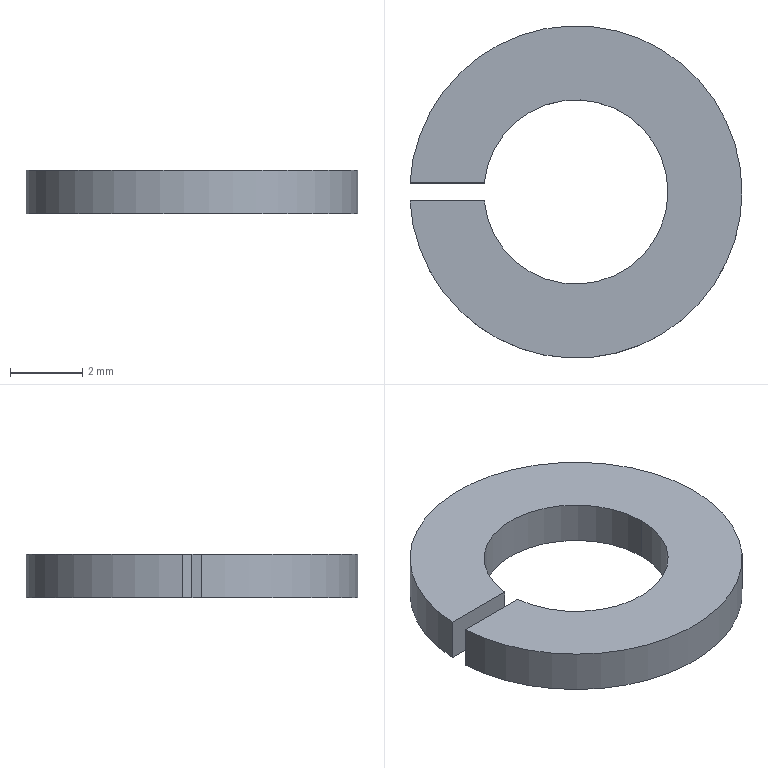Part | SolidWorks | features BaseBody 1 | 1 solid | 8 faces | box 9.193 x 9.2 x 1.2 mm | volume 54.026 mm3 | cylinder 4 | plane 4 | commonest cylinder face diameters 5.1 x2 9.2 x2
STEP:
#1=CARTESIAN_POINT('',(-2.538,0.25,0.));
#2=VERTEX_POINT('',#1);
#3=CARTESIAN_POINT('',(2.55,0.,0.));
#4=VERTEX_POINT('',#3);
#5=CARTESIAN_POINT('',(0.,0.,0.));
#6=DIRECTION('',(0.,0.,-1.));
#7=DIRECTION('',(1.,0.,0.));
#8=AXIS2_PLACEMENT_3D('',#5,#6,#7);
#9=CIRCLE('',#8,2.55);
#10=EDGE_CURVE('',#2,#4,#9,.T.);
#11=ORIENTED_EDGE('',*,*,#10,.T.);
#12=CARTESIAN_POINT('',(2.55,0.,1.2));
#13=VERTEX_POINT('',#12);
#14=CARTESIAN_POINT('',(2.55,0.,1.2));
#15=DIRECTION('',(0.,0.,1.));
#16=VECTOR('',#15,1000.);
#17=LINE('',#14,#16);
#18=EDGE_CURVE('',#4,#13,#17,.T.);
#19=ORIENTED_EDGE('',*,*,#18,.T.);
#20=CARTESIAN_POINT('',(-2.538,0.25,1.2));
#21=VERTEX_POINT('',#20);
#22=CARTESIAN_POINT('',(0.,0.,1.2));
#23=DIRECTION('',(0.,0.,-1.));
#24=DIRECTION('',(1.,0.,0.));
#25=AXIS2_PLACEMENT_3D('',#22,#23,#24);
#26=CIRCLE('',#25,2.55);
#27=EDGE_CURVE('',#21,#13,#26,.T.);
#28=ORIENTED_EDGE('',*,*,#27,.F.);
#29=CARTESIAN_POINT('',(-2.538,0.25,1.2));
#30=DIRECTION('',(0.,0.,1.));
#31=VECTOR('',#30,1000.);
#32=LINE('',#29,#31);
#33=EDGE_CURVE('',#2,#21,#32,.T.);
#34=ORIENTED_EDGE('',*,*,#33,.F.);
#35=EDGE_LOOP('',(#11,#19,#28,#34));
#36=FACE_OUTER_BOUND('',#35,.T.);
#37=CARTESIAN_POINT('',(0.,0.,1.2));
#38=DIRECTION('',(0.,0.,1.));
#39=DIRECTION('',(1.,0.,0.));
#40=AXIS2_PLACEMENT_3D('',#37,#38,#39);
#41=CYLINDRICAL_SURFACE('',#40,2.55);
#42=ADVANCED_FACE('',(#36),#41,.F.);
#43=CARTESIAN_POINT('',(-4.593,-0.25,0.));
#44=VERTEX_POINT('',#43);
#45=CARTESIAN_POINT('',(4.6,0.,0.));
#46=VERTEX_POINT('',#45);
#47=CARTESIAN_POINT('',(0.,0.,0.));
#48=DIRECTION('',(0.,0.,1.));
#49=DIRECTION('',(1.,0.,0.));
#50=AXIS2_PLACEMENT_3D('',#47,#48,#49);
#51=CIRCLE('',#50,4.6);
#52=EDGE_CURVE('',#44,#46,#51,.T.);
#53=ORIENTED_EDGE('',*,*,#52,.T.);
#54=CARTESIAN_POINT('',(4.6,0.,1.2));
#55=VERTEX_POINT('',#54);
#56=CARTESIAN_POINT('',(4.6,0.,1.2));
#57=DIRECTION('',(0.,0.,1.));
#58=VECTOR('',#57,1000.);
#59=LINE('',#56,#58);
#60=EDGE_CURVE('',#46,#55,#59,.T.);
#61=ORIENTED_EDGE('',*,*,#60,.T.);
#62=CARTESIAN_POINT('',(-4.593,-0.25,1.2));
#63=VERTEX_POINT('',#62);
#64=CARTESIAN_POINT('',(0.,0.,1.2));
#65=DIRECTION('',(0.,0.,-1.));
#66=DIRECTION('',(1.,0.,0.));
#67=AXIS2_PLACEMENT_3D('',#64,#65,#66);
#68=CIRCLE('',#67,4.6);
#69=EDGE_CURVE('',#55,#63,#68,.T.);
#70=ORIENTED_EDGE('',*,*,#69,.T.);
#71=CARTESIAN_POINT('',(-4.593,-0.25,1.2));
#72=DIRECTION('',(0.,0.,-1.));
#73=VECTOR('',#72,1000.);
#74=LINE('',#71,#73);
#75=EDGE_CURVE('',#63,#44,#74,.T.);
#76=ORIENTED_EDGE('',*,*,#75,.T.);
#77=EDGE_LOOP('',(#53,#61,#70,#76));
#78=FACE_OUTER_BOUND('',#77,.T.);
#79=CARTESIAN_POINT('',(0.,0.,1.2));
#80=DIRECTION('',(0.,0.,1.));
#81=DIRECTION('',(1.,0.,0.));
#82=AXIS2_PLACEMENT_3D('',#79,#80,#81);
#83=CYLINDRICAL_SURFACE('',#82,4.6);
#84=ADVANCED_FACE('',(#78),#83,.T.);
#85=CARTESIAN_POINT('',(-2.538,-0.25,0.));
#86=VERTEX_POINT('',#85);
#87=CARTESIAN_POINT('',(0.,-0.25,0.));
#88=DIRECTION('',(-1.,0.,0.));
#89=VECTOR('',#88,1000.);
#90=LINE('',#87,#89);
#91=EDGE_CURVE('',#86,#44,#90,.T.);
#92=ORIENTED_EDGE('',*,*,#91,.F.);
#93=CARTESIAN_POINT('',(0.,0.,0.));
#94=DIRECTION('',(0.,0.,-1.));
#95=DIRECTION('',(1.,0.,0.));
#96=AXIS2_PLACEMENT_3D('',#93,#94,#95);
#97=CIRCLE('',#96,2.55);
#98=EDGE_CURVE('',#4,#86,#97,.T.);
#99=ORIENTED_EDGE('',*,*,#98,.F.);
#100=ORIENTED_EDGE('',*,*,#10,.F.);
#101=CARTESIAN_POINT('',(-4.593,0.25,0.));
#102=VERTEX_POINT('',#101);
#103=CARTESIAN_POINT('',(0.,0.25,0.));
#104=DIRECTION('',(1.,0.,0.));
#105=VECTOR('',#104,1000.);
#106=LINE('',#103,#105);
#107=EDGE_CURVE('',#102,#2,#106,.T.);
#108=ORIENTED_EDGE('',*,*,#107,.F.);
#109=CARTESIAN_POINT('',(0.,0.,0.));
#110=DIRECTION('',(0.,0.,1.));
#111=DIRECTION('',(1.,0.,0.));
#112=AXIS2_PLACEMENT_3D('',#109,#110,#111);
#113=CIRCLE('',#112,4.6);
#114=EDGE_CURVE('',#46,#102,#113,.T.);
#115=ORIENTED_EDGE('',*,*,#114,.F.);
#116=ORIENTED_EDGE('',*,*,#52,.F.);
#117=EDGE_LOOP('',(#92,#99,#100,#108,#115,#116));
#118=FACE_OUTER_BOUND('',#117,.T.);
#119=CARTESIAN_POINT('',(0.,0.,0.));
#120=DIRECTION('',(0.,0.,1.));
#121=DIRECTION('',(1.,0.,0.));
#122=AXIS2_PLACEMENT_3D('',#119,#120,#121);
#123=PLANE('',#122);
#124=ADVANCED_FACE('',(#118),#123,.F.);
#125=CARTESIAN_POINT('',(-2.538,-0.25,1.2));
#126=VERTEX_POINT('',#125);
#127=CARTESIAN_POINT('',(-2.538,-0.25,1.2));
#128=DIRECTION('',(-1.,0.,0.));
#129=VECTOR('',#128,1000.);
#130=LINE('',#127,#129);
#131=EDGE_CURVE('',#126,#63,#130,.T.);
#132=ORIENTED_EDGE('',*,*,#131,.F.);
#133=CARTESIAN_POINT('',(-2.538,-0.25,1.2));
#134=DIRECTION('',(0.,0.,1.));
#135=VECTOR('',#134,1000.);
#136=LINE('',#133,#135);
#137=EDGE_CURVE('',#86,#126,#136,.T.);
#138=ORIENTED_EDGE('',*,*,#137,.F.);
#139=ORIENTED_EDGE('',*,*,#91,.T.);
#140=ORIENTED_EDGE('',*,*,#75,.F.);
#141=EDGE_LOOP('',(#132,#138,#139,#140));
#142=FACE_OUTER_BOUND('',#141,.T.);
#143=CARTESIAN_POINT('',(-2.538,-0.25,1.2));
#144=DIRECTION('',(0.,-1.,0.));
#145=DIRECTION('',(0.,0.,-1.));
#146=AXIS2_PLACEMENT_3D('',#143,#144,#145);
#147=PLANE('',#146);
#148=ADVANCED_FACE('',(#142),#147,.F.);
#149=ORIENTED_EDGE('',*,*,#18,.F.);
#150=ORIENTED_EDGE('',*,*,#98,.T.);
#151=ORIENTED_EDGE('',*,*,#137,.T.);
#152=CARTESIAN_POINT('',(0.,0.,1.2));
#153=DIRECTION('',(0.,0.,-1.));
#154=DIRECTION('',(1.,0.,0.));
#155=AXIS2_PLACEMENT_3D('',#152,#153,#154);
#156=CIRCLE('',#155,2.55);
#157=EDGE_CURVE('',#13,#126,#156,.T.);
#158=ORIENTED_EDGE('',*,*,#157,.F.);
#159=EDGE_LOOP('',(#149,#150,#151,#158));
#160=FACE_OUTER_BOUND('',#159,.T.);
#161=CARTESIAN_POINT('',(0.,0.,1.2));
#162=DIRECTION('',(0.,0.,1.));
#163=DIRECTION('',(1.,0.,0.));
#164=AXIS2_PLACEMENT_3D('',#161,#162,#163);
#165=CYLINDRICAL_SURFACE('',#164,2.55);
#166=ADVANCED_FACE('',(#160),#165,.F.);
#167=CARTESIAN_POINT('',(-4.593,0.25,1.2));
#168=VERTEX_POINT('',#167);
#169=CARTESIAN_POINT('',(-4.593,0.25,1.2));
#170=DIRECTION('',(1.,0.,0.));
#171=VECTOR('',#170,1000.);
#172=LINE('',#169,#171);
#173=EDGE_CURVE('',#168,#21,#172,.T.);
#174=ORIENTED_EDGE('',*,*,#173,.F.);
#175=CARTESIAN_POINT('',(-4.593,0.25,1.2));
#176=DIRECTION('',(0.,0.,1.));
#177=VECTOR('',#176,1000.);
#178=LINE('',#175,#177);
#179=EDGE_CURVE('',#102,#168,#178,.T.);
#180=ORIENTED_EDGE('',*,*,#179,.F.);
#181=ORIENTED_EDGE('',*,*,#107,.T.);
#182=ORIENTED_EDGE('',*,*,#33,.T.);
#183=EDGE_LOOP('',(#174,#180,#181,#182));
#184=FACE_OUTER_BOUND('',#183,.T.);
#185=CARTESIAN_POINT('',(-4.593,0.25,1.2));
#186=DIRECTION('',(0.,1.,0.));
#187=DIRECTION('',(0.,0.,1.));
#188=AXIS2_PLACEMENT_3D('',#185,#186,#187);
#189=PLANE('',#188);
#190=ADVANCED_FACE('',(#184),#189,.F.);
#191=ORIENTED_EDGE('',*,*,#60,.F.);
#192=ORIENTED_EDGE('',*,*,#114,.T.);
#193=ORIENTED_EDGE('',*,*,#179,.T.);
#194=CARTESIAN_POINT('',(0.,0.,1.2));
#195=DIRECTION('',(0.,0.,-1.));
#196=DIRECTION('',(1.,0.,0.));
#197=AXIS2_PLACEMENT_3D('',#194,#195,#196);
#198=CIRCLE('',#197,4.6);
#199=EDGE_CURVE('',#168,#55,#198,.T.);
#200=ORIENTED_EDGE('',*,*,#199,.T.);
#201=EDGE_LOOP('',(#191,#192,#193,#200));
#202=FACE_OUTER_BOUND('',#201,.T.);
#203=CARTESIAN_POINT('',(0.,0.,1.2));
#204=DIRECTION('',(0.,0.,1.));
#205=DIRECTION('',(1.,0.,0.));
#206=AXIS2_PLACEMENT_3D('',#203,#204,#205);
#207=CYLINDRICAL_SURFACE('',#206,4.6);
#208=ADVANCED_FACE('',(#202),#207,.T.);
#209=ORIENTED_EDGE('',*,*,#199,.F.);
#210=ORIENTED_EDGE('',*,*,#173,.T.);
#211=ORIENTED_EDGE('',*,*,#27,.T.);
#212=ORIENTED_EDGE('',*,*,#157,.T.);
#213=ORIENTED_EDGE('',*,*,#131,.T.);
#214=ORIENTED_EDGE('',*,*,#69,.F.);
#215=EDGE_LOOP('',(#209,#210,#211,#212,#213,#214));
#216=FACE_OUTER_BOUND('',#215,.T.);
#217=CARTESIAN_POINT('',(0.,0.,1.2));
#218=DIRECTION('',(0.,0.,1.));
#219=DIRECTION('',(1.,0.,0.));
#220=AXIS2_PLACEMENT_3D('',#217,#218,#219);
#221=PLANE('',#220);
#222=ADVANCED_FACE('',(#216),#221,.T.);
#223=CLOSED_SHELL('',(#42,#84,#124,#148,#166,#190,#208,#222));
#224=MANIFOLD_SOLID_BREP('',#223);
#225=CARTESIAN_POINT('',(0.,0.,0.));
#226=DIRECTION('',(0.,0.,1.));
#227=DIRECTION('',(1.,0.,0.));
#228=AXIS2_PLACEMENT_3D('',#225,#226,#227);
#229=(LENGTH_UNIT()NAMED_UNIT(*)SI_UNIT(.MILLI.,.METRE.));
#230=UNCERTAINTY_MEASURE_WITH_UNIT(LENGTH_MEASURE(0.00001),#229,'','');
#231=(NAMED_UNIT(*)PLANE_ANGLE_UNIT()SI_UNIT($,.RADIAN.));
#232=(NAMED_UNIT(*)SI_UNIT($,.STERADIAN.)SOLID_ANGLE_UNIT());
#233=(GEOMETRIC_REPRESENTATION_CONTEXT(3)GLOBAL_UNCERTAINTY_ASSIGNED_CONTEXT((#230))GLOBAL_UNIT_ASSIGNED_CONTEXT((#229,#231,#232))REPRESENTATION_CONTEXT('',''));
#234=ADVANCED_BREP_SHAPE_REPRESENTATION('',(#224,#228),#233);